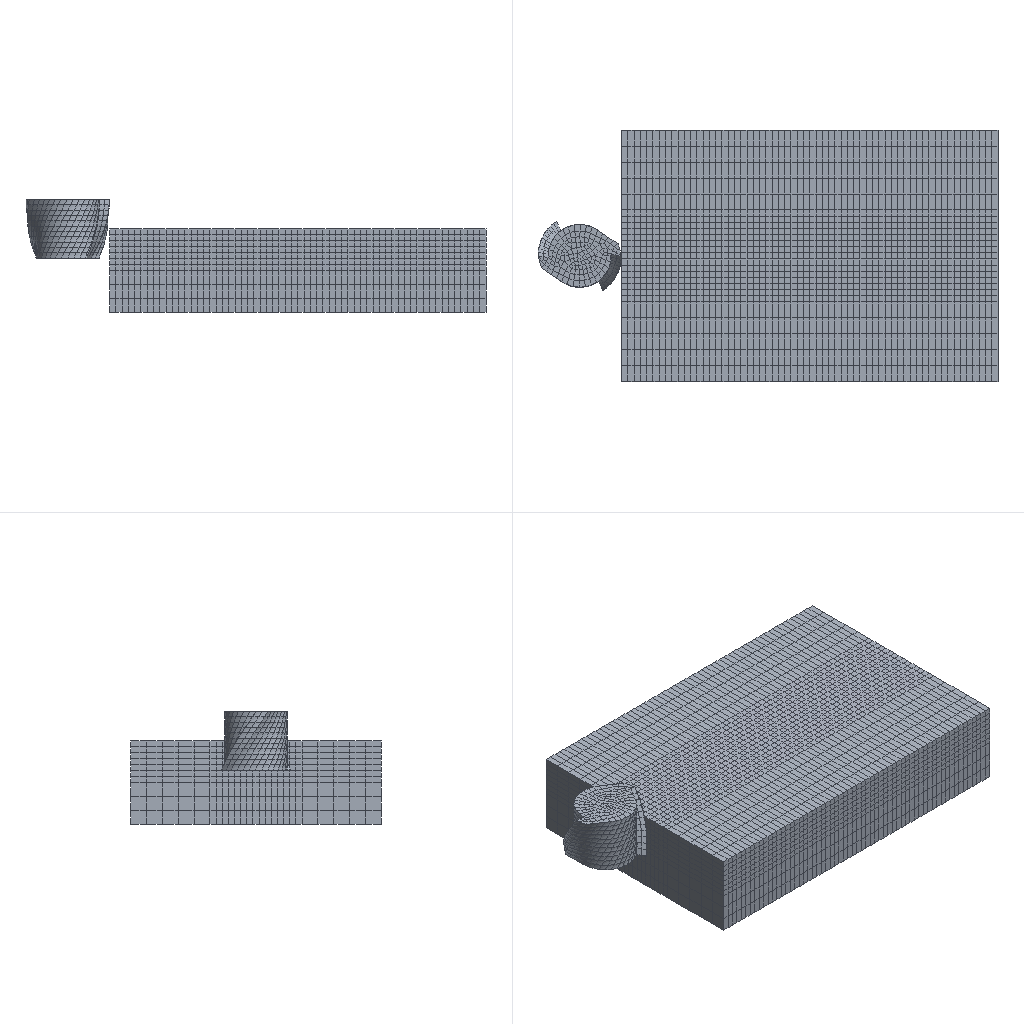Simulation study | abaqus
Set-up summary:
category,name,step,type,value,unit,region
solver,abaqus
solver,version,,,Abaqus/Explicit 2020
units,not stated in the deck,,not stated
analysis,deck,,dynamic temperature-displacement,dynamic temperature-displacement
load_step,Step-1,Step-1,dynamic temperature-displacement
load_step,requested,,,1
mesh,nodes,,,19583
mesh,elements,,,16716
element_type,C3D8RT,,solid,16716
load,load commands in deck,,count,2
bc,support commands in deck,,count,7
material,TOOL,,in results
material,WORK,,in results
check,setup vs results,,match,"per instance, exact: element labels, types and connectivity; labels of the nodes the elements use; coordinates not compared"
Abaqus input file, long lists of numbers shortened:
*Heading
** Job name: Job-1 Model name: Model-1
** Generated by: Abaqus/CAE 2020
*Preprint, echo=NO, model=NO, history=NO, contact=NO
**
** PARTS
**
*Part, name=tool
*Node
      1,   7.573,  0.3525,          14.
      2,   9.922, 0.02249,          14.
** (2134 more lines like these left out)
*Element, type=C3D8RT
   1,    3,  159,  162,   34,  181,  337,  340,  212
   2,   35,    4,   47,   51,  213,  182,  225,  229
** (1714 more lines like these left out)
*Node
   2137,           0.,           0.,           0.
*Nset, nset=tool-RefPt_, internal
2137,
*Nset, nset=Set-2, generate
    1,  2136,     1
*Elset, elset=Set-2, generate
    1,  1716,     1
** Section: tool
*Solid Section, elset=Set-2, material=tool
,
*End Part
**
*Part, name=worka
*Node
      1,           0.,         -41.,          10.
      2,          90.,         -41.,          10.
** (17444 more lines like these left out)
*Element, type=C3D8RT
   1,  320, 2637, 7063, 2581,    1,   25,  929,  170
   2, 2637, 2638, 7064, 7063,   25,   26,  930,  929
** (14998 more lines like these left out)
*Nset, nset=Set-7, generate
     1,  17446,      1
*Elset, elset=Set-7, generate
     1,  15000,      1
** Section: work
*Solid Section, elset=Set-7, material=work
,
*End Part
**
**
** ASSEMBLY
**
*Assembly, name=Assembly
**
*Instance, name=tool-1, part=tool
        -10.,         -30.,          13.
*End Instance
**
*Instance, name=worka-1, part=worka
*End Instance
**
*Nset, nset=Set-4, instance=tool-1
 2137,
*Nset, nset=Set-6, instance=tool-1, generate
    1,  2136,     1
*Elset, elset=Set-6, instance=tool-1, generate
    1,  1716,     1
*Nset, nset=Set-9, instance=tool-1, generate
    1,  2136,     1
*Nset, nset=Set-9, instance=worka-1, generate
     1,  17446,      1
*Elset, elset=Set-9, instance=tool-1, generate
    1,  1716,     1
*Elset, elset=Set-9, instance=worka-1, generate
     1,  15000,      1
*Nset, nset=Set-10, instance=worka-1
    5,    6,    7,    8,    9,   10,   11,   12,   17,   18,   19,   20,   21,   22,   23,   24
  171,  172,  173,  174,  175,  176,  177,  178,  179,  180,  181,  182,  183,  184,  185,  186
** (174 more lines like these left out)
*Elset, elset=Set-10, instance=worka-1
  1801,  1802,  1803,  1804,  1805,  1806,  1807,  1808,  1809,  1810,  1811,  1812,  1813,  1814,  1815,  1816
  1817,  1818,  1819,  1820,  1821,  1822,  1823,  1824,  1825,  1826,  1827,  1828,  1829,  1830,  1831,  1832
** (160 more lines like these left out)
*Nset, nset=b_Set-1, instance=tool-1, generate
    1,  2136,     1
*Elset, elset=b_Set-1, instance=tool-1, generate
    1,  1716,     1
*Nset, nset=s_Set-8, instance=worka-1
     1,     2,     3,     4,    13,    14,    15,    16,    25,    26,    27,    28,    29,    30,    31,    32
    33,    34,    35,    36,    37,    38,    39,    40,    41,    42,    43,    44,    45,    46,    47,    48
** (486 more lines like these left out)
*Elset, elset=s_Set-8, instance=worka-1
    1,    2,    3,    4,    5,    6,    7,    8,    9,   10,   11,   12,   13,   14,   15,   16
   17,   18,   19,   20,   21,   22,   23,   24,   25,   26,   27,   28,   29,   30,   31,   32
** (448 more lines like these left out)
*Nset, nset=s_Set-11, instance=worka-1
     1,     2,     3,     4,    13,    14,    15,    16,    25,    26,    27,    28,    29,    30,    31,    32
    33,    34,    35,    36,    37,    38,    39,    40,    41,    42,    43,    44,    45,    46,    47,    48
** (486 more lines like these left out)
*Elset, elset=s_Set-11, instance=worka-1, generate
 3601,  9900,     1
*Nset, nset=_PickedSet7, internal, instance=tool-1
 2137,
*Elset, elset=_m_Surf-1_S2, internal, instance=tool-1, generate
 1561,  1716,     1
*Elset, elset=_m_Surf-1_S1, internal, instance=tool-1, generate
   1,  156,    1
*Elset, elset=_m_Surf-1_S6, internal, instance=tool-1
    1,   15,   25,   41,   88,   89,  147,  157,  171,  181,  197,  244,  245,  303,  313,  327
  337,  353,  400,  401,  459,  469,  483,  493,  509,  556,  557,  615,  625,  639,  649,  665
** (3 more lines like these left out)
*Elset, elset=_m_Surf-1_S3, internal, instance=tool-1
    2,    6,   13,   17,   29,   33,   38,   40,   49,   51,  110,  111,  146,  148,  149,  150
  158,  162,  169,  173,  185,  189,  194,  196,  205,  207,  266,  267,  302,  304,  305,  306
** (9 more lines like these left out)
*Elset, elset=_m_Surf-1_S5, internal, instance=tool-1
    4,   36,   59,   60,   74,   76,   80,   82,  102,  103,  147,  160,  192,  215,  216,  230
  232,  236,  238,  258,  259,  303,  316,  348,  371,  372,  386,  388,  392,  394,  414,  415
** (6 more lines like these left out)
*Elset, elset=_m_Surf-1_S4, internal, instance=tool-1
   18,   34,   35,  104,  105,  144,  145,  146,  174,  190,  191,  260,  261,  300,  301,  302
  330,  346,  347,  416,  417,  456,  457,  458,  486,  502,  503,  572,  573,  612,  613,  614
** (4 more lines like these left out)
*Surface, type=ELEMENT, name=m_Surf-1
_m_Surf-1_S2, S2
_m_Surf-1_S1, S1
_m_Surf-1_S6, S6
_m_Surf-1_S4, S4
_m_Surf-1_S3, S3
_m_Surf-1_S5, S5
*Elset, elset=_m_Surf-3_S2, internal, instance=tool-1, generate
 1561,  1716,     1
*Elset, elset=_m_Surf-3_S1, internal, instance=tool-1, generate
   1,  156,    1
*Elset, elset=_m_Surf-3_S6, internal, instance=tool-1
    1,   15,   25,   41,   88,   89,  147,  157,  171,  181,  197,  244,  245,  303,  313,  327
  337,  353,  400,  401,  459,  469,  483,  493,  509,  556,  557,  615,  625,  639,  649,  665
** (3 more lines like these left out)
*Elset, elset=_m_Surf-3_S3, internal, instance=tool-1
    2,    6,   13,   17,   29,   33,   38,   40,   49,   51,  110,  111,  146,  148,  149,  150
  158,  162,  169,  173,  185,  189,  194,  196,  205,  207,  266,  267,  302,  304,  305,  306
** (9 more lines like these left out)
*Elset, elset=_m_Surf-3_S5, internal, instance=tool-1
    4,   36,   59,   60,   74,   76,   80,   82,  102,  103,  147,  160,  192,  215,  216,  230
  232,  236,  238,  258,  259,  303,  316,  348,  371,  372,  386,  388,  392,  394,  414,  415
** (6 more lines like these left out)
*Elset, elset=_m_Surf-3_S4, internal, instance=tool-1
   18,   34,   35,  104,  105,  144,  145,  146,  174,  190,  191,  260,  261,  300,  301,  302
  330,  346,  347,  416,  417,  456,  457,  458,  486,  502,  503,  572,  573,  612,  613,  614
** (4 more lines like these left out)
*Surface, type=ELEMENT, name=m_Surf-3
_m_Surf-3_S2, S2
_m_Surf-3_S1, S1
_m_Surf-3_S6, S6
_m_Surf-3_S4, S4
_m_Surf-3_S3, S3
_m_Surf-3_S5, S5
*Elset, elset=_m_Surf-8_S2, internal, instance=tool-1, generate
 1561,  1716,     1
*Elset, elset=_m_Surf-8_S1, internal, instance=tool-1, generate
   1,  156,    1
*Elset, elset=_m_Surf-8_S6, internal, instance=tool-1
    1,   15,   25,   41,   88,   89,  147,  157,  171,  181,  197,  244,  245,  303,  313,  327
  337,  353,  400,  401,  459,  469,  483,  493,  509,  556,  557,  615,  625,  639,  649,  665
** (3 more lines like these left out)
*Elset, elset=_m_Surf-8_S3, internal, instance=tool-1
    2,    6,   13,   17,   29,   33,   38,   40,   49,   51,  110,  111,  146,  148,  149,  150
  158,  162,  169,  173,  185,  189,  194,  196,  205,  207,  266,  267,  302,  304,  305,  306
** (9 more lines like these left out)
*Elset, elset=_m_Surf-8_S5, internal, instance=tool-1
    4,   36,   59,   60,   74,   76,   80,   82,  102,  103,  147,  160,  192,  215,  216,  230
  232,  236,  238,  258,  259,  303,  316,  348,  371,  372,  386,  388,  392,  394,  414,  415
** (6 more lines like these left out)
*Elset, elset=_m_Surf-8_S4, internal, instance=tool-1
   18,   34,   35,  104,  105,  144,  145,  146,  174,  190,  191,  260,  261,  300,  301,  302
  330,  346,  347,  416,  417,  456,  457,  458,  486,  502,  503,  572,  573,  612,  613,  614
** (4 more lines like these left out)
*Surface, type=ELEMENT, name=m_Surf-8
_m_Surf-8_S2, S2
_m_Surf-8_S1, S1
_m_Surf-8_S6, S6
_m_Surf-8_S4, S4
_m_Surf-8_S3, S3
_m_Surf-8_S5, S5
*Elset, elset=_s_Surf-7_S6, internal, instance=worka-1, generate
 3601,  9841,    60
*Elset, elset=_s_Surf-7_S2, internal, instance=worka-1, generate
 9001,  9900,     1
*Elset, elset=_s_Surf-7_S4, internal, instance=worka-1, generate
 3660,  9900,    60
*Surface, type=ELEMENT, name=s_Surf-7
_s_Surf-7_S6, S6
_s_Surf-7_S2, S2
_s_Surf-7_S4, S4
*Surface, type=NODE, name=s_Set-11_CNS_, internal
s_Set-11, 1.
** Constraint: Constraint-1
*Rigid Body, ref node=_PickedSet7, elset=b_Set-1, position=CENTER OF MASS
*End Assembly
**
** MATERIALS
**
*Material, name=tool
*Conductivity
110.,
*Density
 7.8e-09,
*Elastic
210000., 0.3
*Specific Heat
 9.5e+08,
*Material, name=work
*Conductivity
  7.5, 20.
  8.7,200.
 11.8,500.
*Damage Initiation, criterion=JOHNSON COOK
 -0.09,  0.25,  -0.5, 0.014,  3.87, 1650.,   25.,    1.
*Damage Evolution, type=DISPLACEMENT
 0.001,
*Density
 4.4e-09,
*Elastic
108000., 0.33
*Expansion
 9.1e-06, 20.
 9.2e-06,250.
 9.7e-06,500.
*Plastic, hardening=JOHNSON COOK
860., 683., 0.47,   1.,1650.,  25.
*Rate Dependent, type=JOHNSON COOK
 0.035,1.
*Specific Heat
 5.263e+08,
**
** INTERACTION PROPERTIES
**
*Surface Interaction, name=IntProp-1
*Friction
 0.1,
*Surface Behavior, pressure-overclosure=HARD
*Gap Conductance
10.,0.
 0.,1.
**
** PHYSICAL CONSTANTS
**
*Physical Constants, absolute zero=-273., stefan boltzmann=5.67e-08
**
** PREDEFINED FIELDS
**
** Name: Predefined Field-1   Type: Temperature
*Initial Conditions, type=TEMPERATURE
Set-9, 25.
** ----------------------------------------------------------------
**
** STEP: Step-1
**
*Step, name=Step-1, nlgeom=YES
*Dynamic Temperature-displacement, Explicit
, 0.07
*Bulk Viscosity
0.06, 1.2
**
** BOUNDARY CONDITIONS
**
** Name: BC-1 Type: 对称/反对称/完全固定
*Boundary
Set-10, ENCASTRE
** Name: BC-2 Type: 速度/角速度
*Boundary, type=VELOCITY
Set-4, 1, 1, 800.
Set-4, 2, 2
Set-4, 3, 3
Set-4, 4, 4
Set-4, 5, 5
Set-4, 6, 6, 2200.
**
** INTERACTIONS
**
** Interaction: Int-1
*Contact Pair, interaction=IntProp-1, mechanical constraint=KINEMATIC, cpset=Int-1
m_Surf-8, s_Set-11_CNS_
**
** OUTPUT REQUESTS
**
*Restart, write, number interval=1, time marks=NO
**
** FIELD OUTPUT: F-Output-1
**
*Output, field, number interval=100
*Node Output
A, NT, RF, RFL, U, V
*Element Output, directions=YES
E, HFL, LE, MISES, PE, PEEQ, PEEQVAVG, PEVAVG, S, STATUS, SVAVG, TEMP
*Contact Output
CSTRESS,
**
** HISTORY OUTPUT: H-Output-1
**
*Output, history, time interval=1.4e-05
*Node Output, nset=Set-4
RF1, RF2, RF3
*End Step
Results summary:
result,step,Step-1,partial,increments=267675 time=0.05413/0.07
result,analysis,,,"dynamic temperature-displacement, explict"
result,last_loadstep,,,1
result,primary field,,,"U, NT11"
result,reaction total,,FX,71738.551,model units
result,reaction total,,FY,14168.998,model units
result,reaction total,,FZ,-19522.179,model units